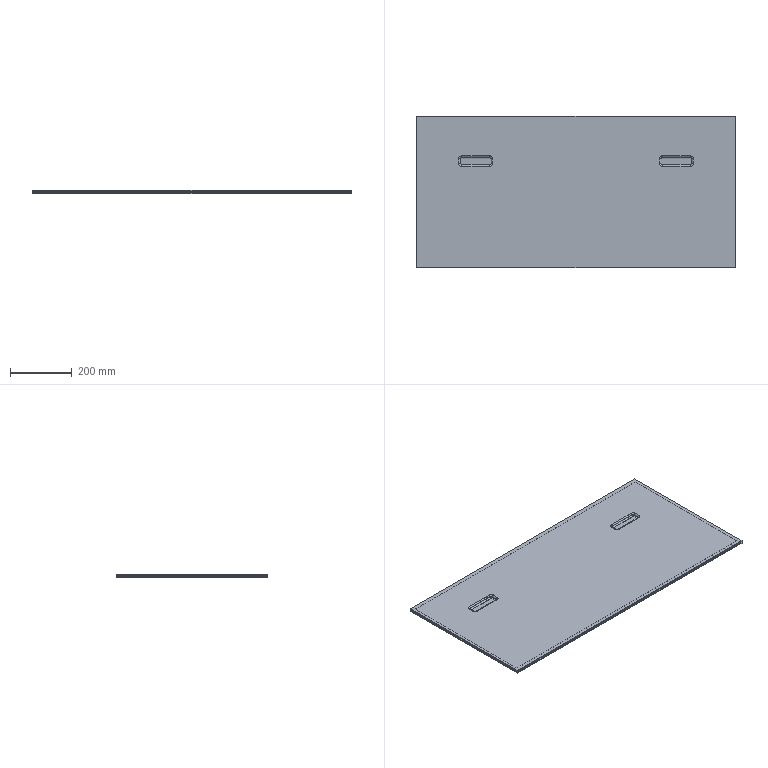Part | NX | 1 solid | 97 faces | box 1030 x 490 x 10 mm | volume 1223683 mm3 | plane 39 | cylinder 34 | torus 24 | commonest cylinder face diameters 10 x16 12 x10 8 x8